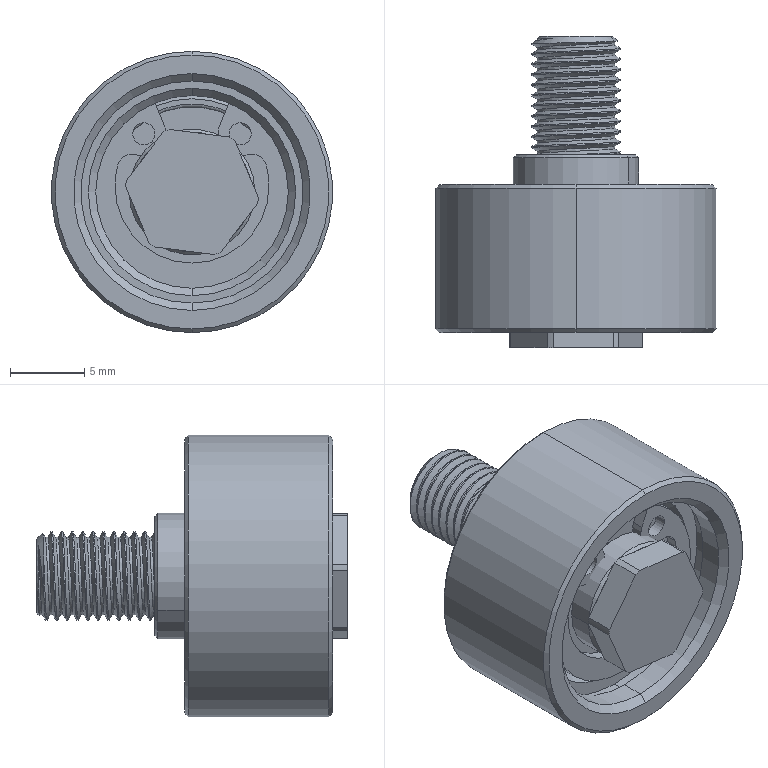Part | NX | features BREP 6 | 6 solids | 147 faces | box 19 x 21 x 19 mm | volume 2699 mm3 | cylinder 70 | plane 30 | cone 29 | torus 16 | spline 2 | commonest cylinder face diameters 6 x26 13 x7 9 x6 1.5 x4 6.1 x4 8.5 x4